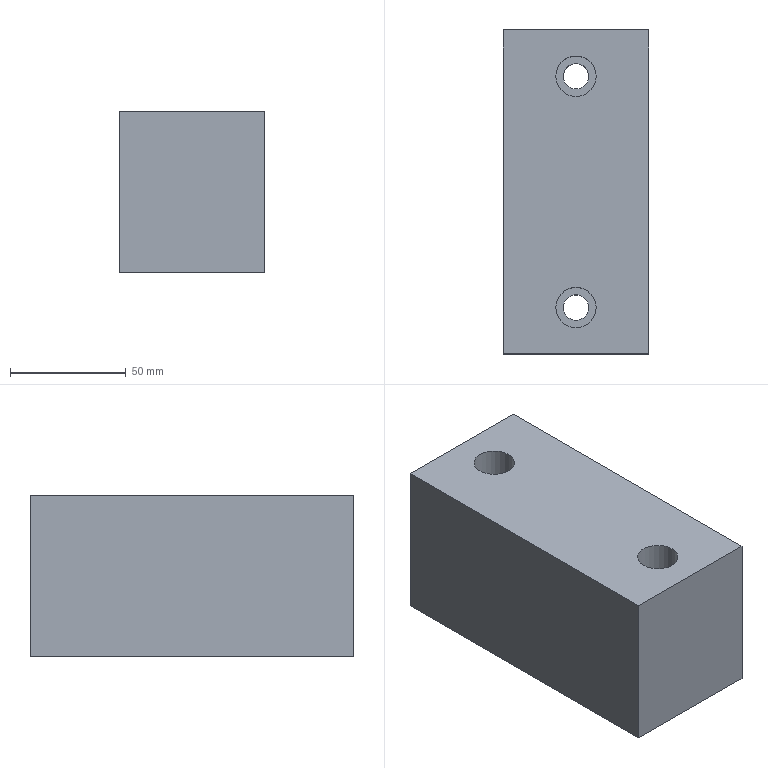Part | NX | features solid 2 | 1 solid | 12 faces | box 63 x 140 x 70 mm | volume 595366 mm3 | plane 8 | cylinder 4 | commonest cylinder face diameters 11 x2 17.5 x2
STEP:
#1=CARTESIAN_POINT('',(1091.5,745.,-125.));
#2=VERTEX_POINT('',#1);
#3=CARTESIAN_POINT('',(1028.5,745.,-125.));
#4=VERTEX_POINT('',#3);
#5=CARTESIAN_POINT('',(1091.5,745.,-125.));
#6=DIRECTION('',(-1.,0.,0.));
#7=VECTOR('',#6,1000.);
#8=LINE('',#5,#7);
#9=EDGE_CURVE('',#2,#4,#8,.T.);
#10=ORIENTED_EDGE('',*,*,#9,.T.);
#11=CARTESIAN_POINT('',(1028.5,745.,-55.));
#12=VERTEX_POINT('',#11);
#13=CARTESIAN_POINT('',(1028.5,745.,-65.));
#14=DIRECTION('',(0.,0.,-1.));
#15=VECTOR('',#14,1000.);
#16=LINE('',#13,#15);
#17=EDGE_CURVE('',#12,#4,#16,.T.);
#18=ORIENTED_EDGE('',*,*,#17,.F.);
#19=CARTESIAN_POINT('',(1091.5,745.,-55.));
#20=VERTEX_POINT('',#19);
#21=CARTESIAN_POINT('',(1091.5,745.,-55.));
#22=DIRECTION('',(-1.,0.,0.));
#23=VECTOR('',#22,1000.);
#24=LINE('',#21,#23);
#25=EDGE_CURVE('',#20,#12,#24,.T.);
#26=ORIENTED_EDGE('',*,*,#25,.F.);
#27=CARTESIAN_POINT('',(1091.5,745.,-65.));
#28=DIRECTION('',(0.,0.,-1.));
#29=VECTOR('',#28,1000.);
#30=LINE('',#27,#29);
#31=EDGE_CURVE('',#20,#2,#30,.T.);
#32=ORIENTED_EDGE('',*,*,#31,.T.);
#33=EDGE_LOOP('',(#10,#18,#26,#32));
#34=FACE_BOUND('',#33,.T.);
#35=CARTESIAN_POINT('',(1091.5,745.,-65.));
#36=DIRECTION('',(0.,1.,0.));
#37=DIRECTION('',(1.,0.,0.));
#38=AXIS2_PLACEMENT_3D('',#35,#36,#37);
#39=PLANE('',#38);
#40=ADVANCED_FACE('',(#34),#39,.T.);
#41=CARTESIAN_POINT('',(1028.5,605.,-125.));
#42=VERTEX_POINT('',#41);
#43=CARTESIAN_POINT('',(1028.5,745.,-125.));
#44=DIRECTION('',(0.,-1.,0.));
#45=VECTOR('',#44,1000.);
#46=LINE('',#43,#45);
#47=EDGE_CURVE('',#4,#42,#46,.T.);
#48=ORIENTED_EDGE('',*,*,#47,.T.);
#49=CARTESIAN_POINT('',(1028.5,605.,-55.));
#50=VERTEX_POINT('',#49);
#51=CARTESIAN_POINT('',(1028.5,605.,-65.));
#52=DIRECTION('',(0.,0.,-1.));
#53=VECTOR('',#52,1000.);
#54=LINE('',#51,#53);
#55=EDGE_CURVE('',#50,#42,#54,.T.);
#56=ORIENTED_EDGE('',*,*,#55,.F.);
#57=CARTESIAN_POINT('',(1028.5,745.,-55.));
#58=DIRECTION('',(0.,-1.,0.));
#59=VECTOR('',#58,1000.);
#60=LINE('',#57,#59);
#61=EDGE_CURVE('',#12,#50,#60,.T.);
#62=ORIENTED_EDGE('',*,*,#61,.F.);
#63=ORIENTED_EDGE('',*,*,#17,.T.);
#64=EDGE_LOOP('',(#48,#56,#62,#63));
#65=FACE_BOUND('',#64,.T.);
#66=CARTESIAN_POINT('',(1028.5,745.,-65.));
#67=DIRECTION('',(-1.,0.,0.));
#68=DIRECTION('',(0.,0.,1.));
#69=AXIS2_PLACEMENT_3D('',#66,#67,#68);
#70=PLANE('',#69);
#71=ADVANCED_FACE('',(#65),#70,.T.);
#72=CARTESIAN_POINT('',(1091.5,605.,-125.));
#73=VERTEX_POINT('',#72);
#74=CARTESIAN_POINT('',(1028.5,605.,-125.));
#75=DIRECTION('',(1.,0.,0.));
#76=VECTOR('',#75,1000.);
#77=LINE('',#74,#76);
#78=EDGE_CURVE('',#42,#73,#77,.T.);
#79=ORIENTED_EDGE('',*,*,#78,.T.);
#80=CARTESIAN_POINT('',(1091.5,605.,-55.));
#81=VERTEX_POINT('',#80);
#82=CARTESIAN_POINT('',(1091.5,605.,-65.));
#83=DIRECTION('',(0.,0.,-1.));
#84=VECTOR('',#83,1000.);
#85=LINE('',#82,#84);
#86=EDGE_CURVE('',#81,#73,#85,.T.);
#87=ORIENTED_EDGE('',*,*,#86,.F.);
#88=CARTESIAN_POINT('',(1091.5,605.,-55.));
#89=DIRECTION('',(1.,0.,0.));
#90=VECTOR('',#89,1000.);
#91=LINE('',#88,#90);
#92=EDGE_CURVE('',#50,#81,#91,.T.);
#93=ORIENTED_EDGE('',*,*,#92,.F.);
#94=ORIENTED_EDGE('',*,*,#55,.T.);
#95=EDGE_LOOP('',(#79,#87,#93,#94));
#96=FACE_BOUND('',#95,.T.);
#97=CARTESIAN_POINT('',(1028.5,605.,-65.));
#98=DIRECTION('',(0.,-1.,0.));
#99=DIRECTION('',(-1.,0.,0.));
#100=AXIS2_PLACEMENT_3D('',#97,#98,#99);
#101=PLANE('',#100);
#102=ADVANCED_FACE('',(#96),#101,.T.);
#103=CARTESIAN_POINT('',(1091.5,745.,-125.));
#104=DIRECTION('',(0.,1.,0.));
#105=VECTOR('',#104,1000.);
#106=LINE('',#103,#105);
#107=EDGE_CURVE('',#73,#2,#106,.T.);
#108=ORIENTED_EDGE('',*,*,#107,.T.);
#109=ORIENTED_EDGE('',*,*,#31,.F.);
#110=CARTESIAN_POINT('',(1091.5,745.,-55.));
#111=DIRECTION('',(0.,1.,0.));
#112=VECTOR('',#111,1000.);
#113=LINE('',#110,#112);
#114=EDGE_CURVE('',#81,#20,#113,.T.);
#115=ORIENTED_EDGE('',*,*,#114,.F.);
#116=ORIENTED_EDGE('',*,*,#86,.T.);
#117=EDGE_LOOP('',(#108,#109,#115,#116));
#118=FACE_BOUND('',#117,.T.);
#119=CARTESIAN_POINT('',(1091.5,625.,-65.));
#120=DIRECTION('',(1.,0.,0.));
#121=DIRECTION('',(0.,-1.,0.));
#122=AXIS2_PLACEMENT_3D('',#119,#120,#121);
#123=PLANE('',#122);
#124=ADVANCED_FACE('',(#118),#123,.T.);
#125=CARTESIAN_POINT('',(1051.25,725.,-55.));
#126=VERTEX_POINT('',#125);
#127=CARTESIAN_POINT('',(1060.,725.,-55.));
#128=DIRECTION('',(0.,0.,1.));
#129=DIRECTION('',(-1.,0.,0.));
#130=AXIS2_PLACEMENT_3D('',#127,#128,#129);
#131=CIRCLE('',#130,8.75);
#132=EDGE_CURVE('',#126,#126,#131,.F.);
#133=ORIENTED_EDGE('',*,*,#132,.T.);
#134=EDGE_LOOP('',(#133));
#135=FACE_BOUND('',#134,.T.);
#136=CARTESIAN_POINT('',(1051.25,625.,-55.));
#137=VERTEX_POINT('',#136);
#138=CARTESIAN_POINT('',(1060.,625.,-55.));
#139=DIRECTION('',(0.,0.,1.));
#140=DIRECTION('',(-1.,0.,0.));
#141=AXIS2_PLACEMENT_3D('',#138,#139,#140);
#142=CIRCLE('',#141,8.75);
#143=EDGE_CURVE('',#137,#137,#142,.T.);
#144=ORIENTED_EDGE('',*,*,#143,.F.);
#145=EDGE_LOOP('',(#144));
#146=FACE_BOUND('',#145,.T.);
#147=ORIENTED_EDGE('',*,*,#25,.T.);
#148=ORIENTED_EDGE('',*,*,#61,.T.);
#149=ORIENTED_EDGE('',*,*,#92,.T.);
#150=ORIENTED_EDGE('',*,*,#114,.T.);
#151=EDGE_LOOP('',(#147,#148,#149,#150));
#152=FACE_BOUND('',#151,.T.);
#153=CARTESIAN_POINT('',(1091.5,745.,-55.));
#154=DIRECTION('',(0.,0.,1.));
#155=DIRECTION('',(0.,-1.,0.));
#156=AXIS2_PLACEMENT_3D('',#153,#154,#155);
#157=PLANE('',#156);
#158=ADVANCED_FACE('',(#135,#146,#152),#157,.T.);
#159=CARTESIAN_POINT('',(1054.5,725.,-125.));
#160=VERTEX_POINT('',#159);
#161=CARTESIAN_POINT('',(1060.,725.,-125.));
#162=DIRECTION('',(0.,0.,1.));
#163=DIRECTION('',(-1.,0.,0.));
#164=AXIS2_PLACEMENT_3D('',#161,#162,#163);
#165=CIRCLE('',#164,5.5);
#166=EDGE_CURVE('',#160,#160,#165,.F.);
#167=ORIENTED_EDGE('',*,*,#166,.F.);
#168=EDGE_LOOP('',(#167));
#169=FACE_BOUND('',#168,.T.);
#170=CARTESIAN_POINT('',(1054.5,625.,-125.));
#171=VERTEX_POINT('',#170);
#172=CARTESIAN_POINT('',(1060.,625.,-125.));
#173=DIRECTION('',(0.,0.,1.));
#174=DIRECTION('',(-1.,0.,0.));
#175=AXIS2_PLACEMENT_3D('',#172,#173,#174);
#176=CIRCLE('',#175,5.5);
#177=EDGE_CURVE('',#171,#171,#176,.F.);
#178=ORIENTED_EDGE('',*,*,#177,.F.);
#179=EDGE_LOOP('',(#178));
#180=FACE_BOUND('',#179,.T.);
#181=ORIENTED_EDGE('',*,*,#9,.F.);
#182=ORIENTED_EDGE('',*,*,#107,.F.);
#183=ORIENTED_EDGE('',*,*,#78,.F.);
#184=ORIENTED_EDGE('',*,*,#47,.F.);
#185=EDGE_LOOP('',(#181,#182,#183,#184));
#186=FACE_BOUND('',#185,.T.);
#187=CARTESIAN_POINT('',(1091.5,745.,-125.));
#188=DIRECTION('',(0.,0.,1.));
#189=DIRECTION('',(0.,-1.,0.));
#190=AXIS2_PLACEMENT_3D('',#187,#188,#189);
#191=PLANE('',#190);
#192=ADVANCED_FACE('',(#169,#180,#186),#191,.F.);
#193=CARTESIAN_POINT('',(1065.5,625.,-85.));
#194=VERTEX_POINT('',#193);
#195=CARTESIAN_POINT('',(1060.,625.,-85.));
#196=DIRECTION('',(0.,0.,-1.));
#197=DIRECTION('',(1.,0.,0.));
#198=AXIS2_PLACEMENT_3D('',#195,#196,#197);
#199=CIRCLE('',#198,5.5);
#200=EDGE_CURVE('',#194,#194,#199,.F.);
#201=ORIENTED_EDGE('',*,*,#200,.T.);
#202=EDGE_LOOP('',(#201));
#203=FACE_BOUND('',#202,.T.);
#204=ORIENTED_EDGE('',*,*,#177,.T.);
#205=EDGE_LOOP('',(#204));
#206=FACE_BOUND('',#205,.T.);
#207=CARTESIAN_POINT('',(1060.,625.,-145.));
#208=DIRECTION('',(0.,0.,-1.));
#209=DIRECTION('',(0.,1.,0.));
#210=AXIS2_PLACEMENT_3D('',#207,#208,#209);
#211=CYLINDRICAL_SURFACE('',#210,5.5);
#212=ADVANCED_FACE('',(#203,#206),#211,.F.);
#213=ORIENTED_EDGE('',*,*,#200,.F.);
#214=EDGE_LOOP('',(#213));
#215=FACE_BOUND('',#214,.T.);
#216=CARTESIAN_POINT('',(1068.75,625.,-85.));
#217=VERTEX_POINT('',#216);
#218=CARTESIAN_POINT('',(1060.,625.,-85.));
#219=DIRECTION('',(0.,0.,-1.));
#220=DIRECTION('',(1.,0.,0.));
#221=AXIS2_PLACEMENT_3D('',#218,#219,#220);
#222=CIRCLE('',#221,8.75);
#223=EDGE_CURVE('',#217,#217,#222,.F.);
#224=ORIENTED_EDGE('',*,*,#223,.T.);
#225=EDGE_LOOP('',(#224));
#226=FACE_BOUND('',#225,.T.);
#227=CARTESIAN_POINT('',(1060.,625.,-85.));
#228=DIRECTION('',(0.,0.,-1.));
#229=DIRECTION('',(0.,1.,0.));
#230=AXIS2_PLACEMENT_3D('',#227,#228,#229);
#231=PLANE('',#230);
#232=ADVANCED_FACE('',(#215,#226),#231,.F.);
#233=ORIENTED_EDGE('',*,*,#223,.F.);
#234=EDGE_LOOP('',(#233));
#235=FACE_BOUND('',#234,.T.);
#236=ORIENTED_EDGE('',*,*,#143,.T.);
#237=EDGE_LOOP('',(#236));
#238=FACE_BOUND('',#237,.T.);
#239=CARTESIAN_POINT('',(1060.,625.,-65.));
#240=DIRECTION('',(0.,0.,-1.));
#241=DIRECTION('',(0.,1.,0.));
#242=AXIS2_PLACEMENT_3D('',#239,#240,#241);
#243=CYLINDRICAL_SURFACE('',#242,8.75);
#244=ADVANCED_FACE('',(#235,#238),#243,.F.);
#245=CARTESIAN_POINT('',(1065.5,725.,-85.));
#246=VERTEX_POINT('',#245);
#247=CARTESIAN_POINT('',(1060.,725.,-85.));
#248=DIRECTION('',(0.,0.,-1.));
#249=DIRECTION('',(1.,0.,0.));
#250=AXIS2_PLACEMENT_3D('',#247,#248,#249);
#251=CIRCLE('',#250,5.5);
#252=EDGE_CURVE('',#246,#246,#251,.T.);
#253=ORIENTED_EDGE('',*,*,#252,.F.);
#254=EDGE_LOOP('',(#253));
#255=FACE_BOUND('',#254,.T.);
#256=ORIENTED_EDGE('',*,*,#166,.T.);
#257=EDGE_LOOP('',(#256));
#258=FACE_BOUND('',#257,.T.);
#259=CARTESIAN_POINT('',(1060.,725.,-145.));
#260=DIRECTION('',(0.,0.,-1.));
#261=DIRECTION('',(0.,-1.,0.));
#262=AXIS2_PLACEMENT_3D('',#259,#260,#261);
#263=CYLINDRICAL_SURFACE('',#262,5.5);
#264=ADVANCED_FACE('',(#255,#258),#263,.F.);
#265=ORIENTED_EDGE('',*,*,#252,.T.);
#266=EDGE_LOOP('',(#265));
#267=FACE_BOUND('',#266,.T.);
#268=CARTESIAN_POINT('',(1068.75,725.,-85.));
#269=VERTEX_POINT('',#268);
#270=CARTESIAN_POINT('',(1060.,725.,-85.));
#271=DIRECTION('',(0.,0.,-1.));
#272=DIRECTION('',(1.,0.,0.));
#273=AXIS2_PLACEMENT_3D('',#270,#271,#272);
#274=CIRCLE('',#273,8.75);
#275=EDGE_CURVE('',#269,#269,#274,.T.);
#276=ORIENTED_EDGE('',*,*,#275,.F.);
#277=EDGE_LOOP('',(#276));
#278=FACE_BOUND('',#277,.T.);
#279=CARTESIAN_POINT('',(1060.,725.,-85.));
#280=DIRECTION('',(0.,0.,-1.));
#281=DIRECTION('',(0.,-1.,0.));
#282=AXIS2_PLACEMENT_3D('',#279,#280,#281);
#283=PLANE('',#282);
#284=ADVANCED_FACE('',(#267,#278),#283,.F.);
#285=ORIENTED_EDGE('',*,*,#275,.T.);
#286=EDGE_LOOP('',(#285));
#287=FACE_BOUND('',#286,.T.);
#288=ORIENTED_EDGE('',*,*,#132,.F.);
#289=EDGE_LOOP('',(#288));
#290=FACE_BOUND('',#289,.T.);
#291=CARTESIAN_POINT('',(1060.,725.,-65.));
#292=DIRECTION('',(0.,0.,-1.));
#293=DIRECTION('',(0.,-1.,0.));
#294=AXIS2_PLACEMENT_3D('',#291,#292,#293);
#295=CYLINDRICAL_SURFACE('',#294,8.75);
#296=ADVANCED_FACE('',(#287,#290),#295,.F.);
#297=CLOSED_SHELL('',(#40,#71,#102,#124,#158,#192,#212,#232,#244,#264,#284,#296));
#298=MANIFOLD_SOLID_BREP('',#297);
#299=(LENGTH_UNIT()NAMED_UNIT(*)SI_UNIT(.MILLI.,.METRE.));
#300=UNCERTAINTY_MEASURE_WITH_UNIT(LENGTH_MEASURE(0.00001),#299,'','');
#301=(NAMED_UNIT(*)PLANE_ANGLE_UNIT()SI_UNIT($,.RADIAN.));
#302=(NAMED_UNIT(*)SI_UNIT($,.STERADIAN.)SOLID_ANGLE_UNIT());
#303=(GEOMETRIC_REPRESENTATION_CONTEXT(3)GLOBAL_UNCERTAINTY_ASSIGNED_CONTEXT((#300))GLOBAL_UNIT_ASSIGNED_CONTEXT((#299,#301,#302))REPRESENTATION_CONTEXT('',''));
#304=ADVANCED_BREP_SHAPE_REPRESENTATION('',(#298),#303);